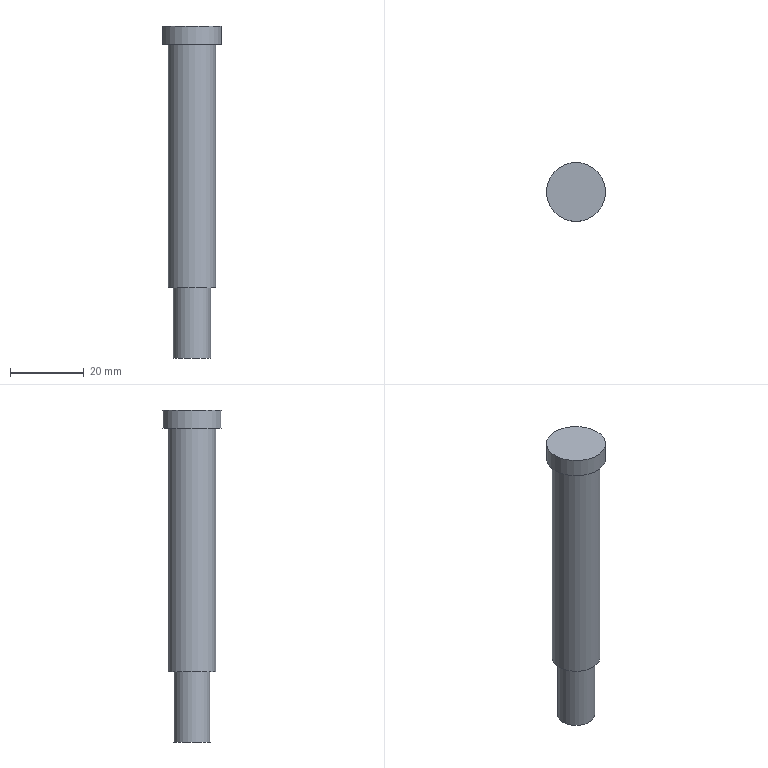Part | NX | features solid 2 | 1 solid | 7 faces | box 16 x 16 x 90 mm | volume 11288 mm3 | plane 4 | cylinder 3 | commonest cylinder face diameters 10.1 x1 13 x1 16 x1
STEP:
#1=CARTESIAN_POINT('',(-150.931,-669.725,29.));
#2=VERTEX_POINT('',#1);
#3=CARTESIAN_POINT('',(-157.431,-669.725,29.));
#4=DIRECTION('',(0.,0.,1.));
#5=DIRECTION('',(1.,0.,0.));
#6=AXIS2_PLACEMENT_3D('',#3,#4,#5);
#7=CIRCLE('',#6,6.5);
#8=EDGE_CURVE('',#2,#2,#7,.T.);
#9=ORIENTED_EDGE('',*,*,#8,.T.);
#10=EDGE_LOOP('',(#9));
#11=FACE_BOUND('',#10,.T.);
#12=CARTESIAN_POINT('',(-150.931,-669.725,95.));
#13=VERTEX_POINT('',#12);
#14=CARTESIAN_POINT('',(-157.431,-669.725,95.));
#15=DIRECTION('',(0.,0.,1.));
#16=DIRECTION('',(1.,0.,0.));
#17=AXIS2_PLACEMENT_3D('',#14,#15,#16);
#18=CIRCLE('',#17,6.5);
#19=EDGE_CURVE('',#13,#13,#18,.T.);
#20=ORIENTED_EDGE('',*,*,#19,.F.);
#21=EDGE_LOOP('',(#20));
#22=FACE_BOUND('',#21,.T.);
#23=CARTESIAN_POINT('',(-157.431,-669.725,100.));
#24=DIRECTION('',(0.,0.,-1.));
#25=DIRECTION('',(-1.,0.,0.));
#26=AXIS2_PLACEMENT_3D('',#23,#24,#25);
#27=CYLINDRICAL_SURFACE('',#26,6.5);
#28=ADVANCED_FACE('',(#11,#22),#27,.T.);
#29=CARTESIAN_POINT('',(-152.381,-669.725,29.));
#30=VERTEX_POINT('',#29);
#31=CARTESIAN_POINT('',(-157.431,-669.725,29.));
#32=DIRECTION('',(0.,0.,1.));
#33=DIRECTION('',(1.,0.,0.));
#34=AXIS2_PLACEMENT_3D('',#31,#32,#33);
#35=CIRCLE('',#34,5.05);
#36=EDGE_CURVE('',#30,#30,#35,.T.);
#37=ORIENTED_EDGE('',*,*,#36,.T.);
#38=EDGE_LOOP('',(#37));
#39=FACE_BOUND('',#38,.T.);
#40=ORIENTED_EDGE('',*,*,#8,.F.);
#41=EDGE_LOOP('',(#40));
#42=FACE_BOUND('',#41,.T.);
#43=CARTESIAN_POINT('',(-157.431,-669.725,29.));
#44=DIRECTION('',(0.,0.,1.));
#45=DIRECTION('',(1.,0.,0.));
#46=AXIS2_PLACEMENT_3D('',#43,#44,#45);
#47=PLANE('',#46);
#48=ADVANCED_FACE('',(#39,#42),#47,.F.);
#49=CARTESIAN_POINT('',(-149.431,-669.725,95.));
#50=VERTEX_POINT('',#49);
#51=CARTESIAN_POINT('',(-157.431,-669.725,95.));
#52=DIRECTION('',(0.,0.,1.));
#53=DIRECTION('',(1.,0.,0.));
#54=AXIS2_PLACEMENT_3D('',#51,#52,#53);
#55=CIRCLE('',#54,8.);
#56=EDGE_CURVE('',#50,#50,#55,.T.);
#57=ORIENTED_EDGE('',*,*,#56,.F.);
#58=EDGE_LOOP('',(#57));
#59=FACE_BOUND('',#58,.T.);
#60=ORIENTED_EDGE('',*,*,#19,.T.);
#61=EDGE_LOOP('',(#60));
#62=FACE_BOUND('',#61,.T.);
#63=CARTESIAN_POINT('',(-157.431,-669.725,95.));
#64=DIRECTION('',(0.,0.,1.));
#65=DIRECTION('',(1.,0.,0.));
#66=AXIS2_PLACEMENT_3D('',#63,#64,#65);
#67=PLANE('',#66);
#68=ADVANCED_FACE('',(#59,#62),#67,.F.);
#69=ORIENTED_EDGE('',*,*,#56,.T.);
#70=EDGE_LOOP('',(#69));
#71=FACE_BOUND('',#70,.T.);
#72=CARTESIAN_POINT('',(-149.431,-669.725,100.));
#73=VERTEX_POINT('',#72);
#74=CARTESIAN_POINT('',(-157.431,-669.725,100.));
#75=DIRECTION('',(0.,0.,1.));
#76=DIRECTION('',(1.,0.,0.));
#77=AXIS2_PLACEMENT_3D('',#74,#75,#76);
#78=CIRCLE('',#77,8.);
#79=EDGE_CURVE('',#73,#73,#78,.T.);
#80=ORIENTED_EDGE('',*,*,#79,.F.);
#81=EDGE_LOOP('',(#80));
#82=FACE_BOUND('',#81,.T.);
#83=CARTESIAN_POINT('',(-157.431,-669.725,95.));
#84=DIRECTION('',(0.,0.,1.));
#85=DIRECTION('',(1.,0.,0.));
#86=AXIS2_PLACEMENT_3D('',#83,#84,#85);
#87=CYLINDRICAL_SURFACE('',#86,8.);
#88=ADVANCED_FACE('',(#71,#82),#87,.T.);
#89=ORIENTED_EDGE('',*,*,#79,.T.);
#90=EDGE_LOOP('',(#89));
#91=FACE_BOUND('',#90,.T.);
#92=CARTESIAN_POINT('',(-157.431,-669.725,100.));
#93=DIRECTION('',(0.,0.,1.));
#94=DIRECTION('',(1.,0.,0.));
#95=AXIS2_PLACEMENT_3D('',#92,#93,#94);
#96=PLANE('',#95);
#97=ADVANCED_FACE('',(#91),#96,.T.);
#98=CARTESIAN_POINT('',(-152.381,-669.725,10.));
#99=VERTEX_POINT('',#98);
#100=CARTESIAN_POINT('',(-157.431,-669.725,10.));
#101=DIRECTION('',(0.,0.,1.));
#102=DIRECTION('',(1.,0.,0.));
#103=AXIS2_PLACEMENT_3D('',#100,#101,#102);
#104=CIRCLE('',#103,5.05);
#105=EDGE_CURVE('',#99,#99,#104,.T.);
#106=ORIENTED_EDGE('',*,*,#105,.T.);
#107=EDGE_LOOP('',(#106));
#108=FACE_BOUND('',#107,.T.);
#109=ORIENTED_EDGE('',*,*,#36,.F.);
#110=EDGE_LOOP('',(#109));
#111=FACE_BOUND('',#110,.T.);
#112=CARTESIAN_POINT('',(-157.431,-669.725,10.));
#113=DIRECTION('',(0.,0.,1.));
#114=DIRECTION('',(1.,0.,0.));
#115=AXIS2_PLACEMENT_3D('',#112,#113,#114);
#116=CYLINDRICAL_SURFACE('',#115,5.05);
#117=ADVANCED_FACE('',(#108,#111),#116,.T.);
#118=ORIENTED_EDGE('',*,*,#105,.F.);
#119=EDGE_LOOP('',(#118));
#120=FACE_BOUND('',#119,.T.);
#121=CARTESIAN_POINT('',(-157.431,-669.725,10.));
#122=DIRECTION('',(0.,0.,1.));
#123=DIRECTION('',(1.,0.,0.));
#124=AXIS2_PLACEMENT_3D('',#121,#122,#123);
#125=PLANE('',#124);
#126=ADVANCED_FACE('',(#120),#125,.F.);
#127=CLOSED_SHELL('',(#28,#48,#68,#88,#97,#117,#126));
#128=MANIFOLD_SOLID_BREP('',#127);
#129=(LENGTH_UNIT()NAMED_UNIT(*)SI_UNIT(.MILLI.,.METRE.));
#130=UNCERTAINTY_MEASURE_WITH_UNIT(LENGTH_MEASURE(0.00001),#129,'','');
#131=(NAMED_UNIT(*)PLANE_ANGLE_UNIT()SI_UNIT($,.RADIAN.));
#132=(NAMED_UNIT(*)SI_UNIT($,.STERADIAN.)SOLID_ANGLE_UNIT());
#133=(GEOMETRIC_REPRESENTATION_CONTEXT(3)GLOBAL_UNCERTAINTY_ASSIGNED_CONTEXT((#130))GLOBAL_UNIT_ASSIGNED_CONTEXT((#129,#131,#132))REPRESENTATION_CONTEXT('',''));
#134=ADVANCED_BREP_SHAPE_REPRESENTATION('',(#128),#133);